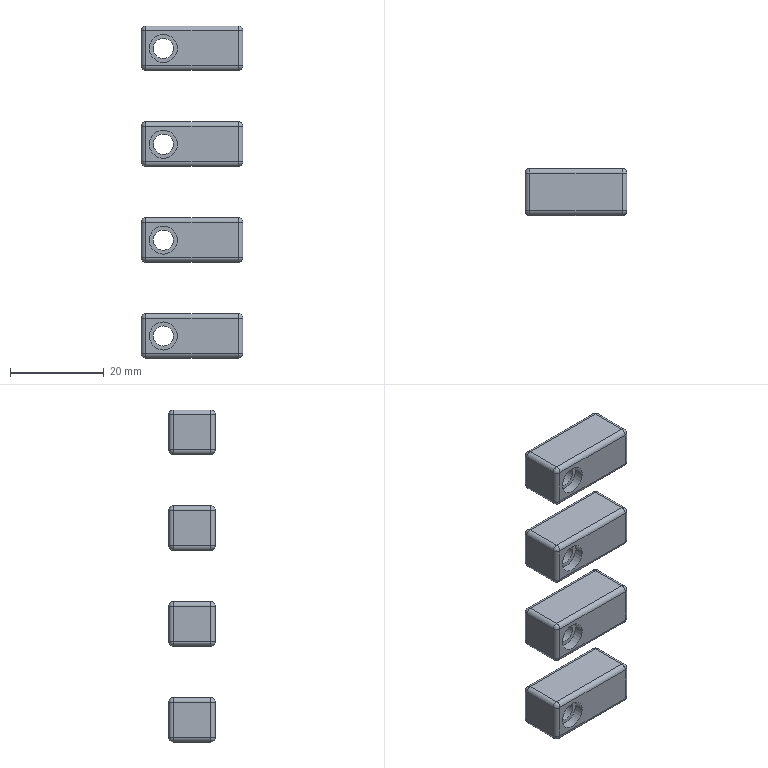Part | 4 solids | 132 faces | box 21.75 x 10 x 71 mm | volume 6905 mm3 | cylinder 60 | plane 40 | sphere 32 | commonest cylinder face diameters 2 x48 4.3 x4 6 x4 7.8 x4